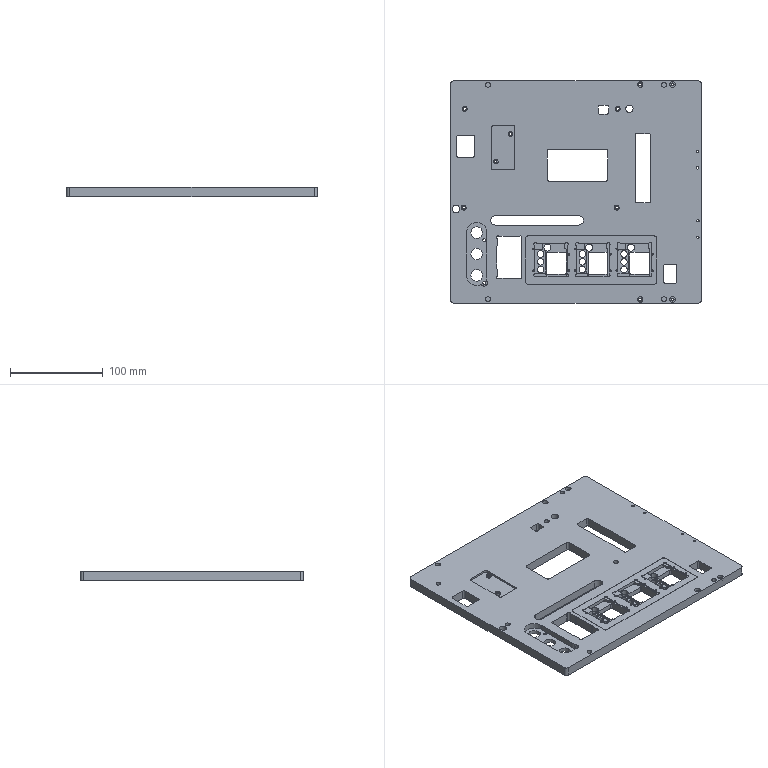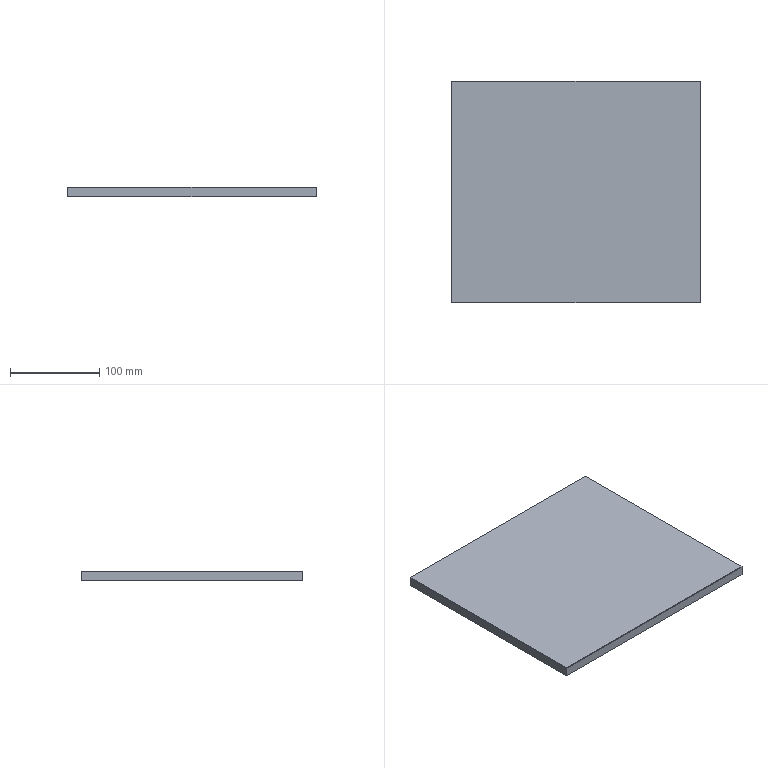CAM job | NX | 3-axis milling, drilling | part box 270 x 240 x 10 mm | stock box 278 x 248 x 11 mm
Tools:
number,name,description,diameter,corner_radius,flute_length,length,flutes
1,D6A45,Milling Tool-5 Parameters,6.0,0.0,3.0,3.0,2
23,3.2ZT,Drilling Tool,3.2,0.0,35.0,50.0,2
11,2.6ZT,Drilling Tool,2.6,0.0,35.0,50.0,2
12,5.2ZT,Drilling Tool,5.2,0.0,35.0,50.0,2
13,1.6ZT,Drilling Tool,1.6,0.0,35.0,50.0,2
4,D10,Milling Tool-5 Parameters,10.0,0.0,50.0,75.0,2
16,D6JING,Milling Tool-5 Parameters,6.0,0.0,50.0,75.0,2
17,D3,Milling Tool-5 Parameters,3.0,0.0,50.0,75.0,2
18,D2,Milling Tool-5 Parameters,2.0,0.0,50.0,75.0,2
3,D63,Milling Tool-5 Parameters,63.0,0.0,50.0,75.0,2
Operations:
program,operation,operation_type,tool,method,geometry_group,spindle_rpm,surface_speed,feed_per_tooth,feed_cut,feed_plunge,cut_length_mm,path_length_mm,cut_time_min,machine_time_min
1夹,11_COPY,ZLevelMilling,D6A45,METHOD,B,9500.0,179.0,0.0526,1000.0,100.0,2532.317,9979.461,2.532,3.277
1夹,11_COPY_COPY,ZLevelMilling,D6A45,METHOD,B,9500.0,179.0,0.0526,1000.0,100.0,494.985,866.892,0.495,0.5322
1夹,ADAPTIVE_MILLING_COPY,CavityMilling,D10,METHOD,B,9500.0,298.0,0.1842,3500.0,1000.0,4240.976,4316.976,1.212,1.22
1夹,ZLEVEL_PROFILE_1_COPY,ZLevelMilling,D6JING,METHOD,B,9500.0,298.0,0.0526,1000.0,100.0,1037.609,1115.609,1.038,1.045
1夹,HOLE_MILLING_COPY_2,CylinderMilling,D2,METHOD,B,9500.0,59.0,0.0579,1100.0,100.0,640.058,1392.794,0.5819,0.6571
2夹,FLOOR_WALL,VolumeBased25DMillingOperation,D63,METHOD,A,6500.0,1286.0,0.0962,1250.0,100.0,11123.775,12232.039,8.899,9.01
2夹,DRILLING_COPY_1,Operation,D6A45,METHOD,A,5000.0,94.0,0.025,250.0,0.0,176.4,1685.811,0.7056,0.8565
2夹,DRILLING_COPY_1_COPY,Operation,3.2ZT,METHOD,A,2000.0,20.0,0.0625,250.0,0.0,169.614,1118.318,0.6785,0.7733
2夹,DRILLING_COPY_1_COPY_COPY,Operation,2.6ZT,METHOD,A,2000.0,16.0,0.05,200.0,0.0,100.687,606.395,0.5034,0.554
2夹,DRILLING_COPY_1_COPY_COPY_COPY,Operation,5.2ZT,METHOD,A,2000.0,16.0,0.05,200.0,0.0,42.249,764.565,0.2112,0.2835
2夹,DRILLING_COPY_1_COPY_COPY_COPY_COPY,Operation,1.6ZT,METHOD,A,2000.0,10.0,0.0375,150.0,0.0,137.768,602.756,0.9185,0.965
2夹,11,ZLevelMilling,D6A45,METHOD,A,9500.0,179.0,0.0526,1000.0,100.0,3193.76,9745.818,3.194,3.849
2夹,FLOOR_WALL_COPY,VolumeBased25DMillingOperation,D63,METHOD,A,6500.0,1286.0,0.0962,1250.0,100.0,2224.785,2278.785,1.78,1.785
2夹,ADAPTIVE_MILLING,CavityMilling,D10,METHOD,A,9500.0,298.0,0.1842,3500.0,1000.0,20879.622,22846.933,9.864,10.061
2夹,ZLEVEL_PROFILE,ZLevelMilling,D10,METHOD,A,9500.0,298.0,0.1579,3000.0,1000.0,1861.742,2138.405,0.6715,0.6992
2夹,HOLE_MILLING_COPY,CylinderMilling,D10,METHOD,A,9500.0,0.0,0.0,1650.0,100.0,136.608,409.108,0.0828,0.11
2夹,ZLEVEL_PROFILE_COPY,ZLevelMilling,D6JING,METHOD,A,9500.0,179.0,0.1053,2000.0,1000.0,4288.755,4574.997,2.173,2.202
2夹,ZLEVEL_PROFILE_COPY_COPY,ZLevelMilling,D6JING,METHOD,A,9500.0,179.0,0.1053,2000.0,1000.0,629.968,925.024,0.358,0.3875
2夹,ZLEVEL_PROFILE_COPY_COPY_COPY_1,ZLevelMilling,D6JING,METHOD,A,9500.0,179.0,0.1053,2000.0,1000.0,5224.756,14593.317,3.19,4.127
2夹,HOLE_MILLING,CylinderMilling,D6JING,METHOD,A,9500.0,0.0,0.0,1650.0,100.0,790.148,2258.076,0.4789,0.6257
2夹,ZLEVEL_PROFILE_1,ZLevelMilling,D6JING,METHOD,A,9500.0,298.0,0.0526,1000.0,100.0,1271.976,7168.785,1.272,1.862
2夹,FLOOR_WALL_1_COPY_1,VolumeBased25DMillingOperation,D6JING,METHOD,A,9500.0,298.0,0.0632,1200.0,1000.0,4366.477,6178.86,3.661,3.848
2夹,ZLEVEL_PROFILE_COPY_COPY_COPY_1_COPY,ZLevelMilling,D3,METHOD,A,9500.0,89.0,0.0789,1500.0,1000.0,6902.942,18490.224,4.975,6.134
2夹,HOLE_MILLING_COPY_1,CylinderMilling,D3,METHOD,A,9500.0,89.0,0.0684,1300.0,100.0,927.05,2066.009,0.7131,0.827
2夹,ZLEVEL_PROFILE_COPY_COPY_COPY_1_COPY_COPY,ZLevelMilling,D2,METHOD,A,9500.0,59.0,0.0632,1200.0,1000.0,2647.797,10186.685,2.288,3.042